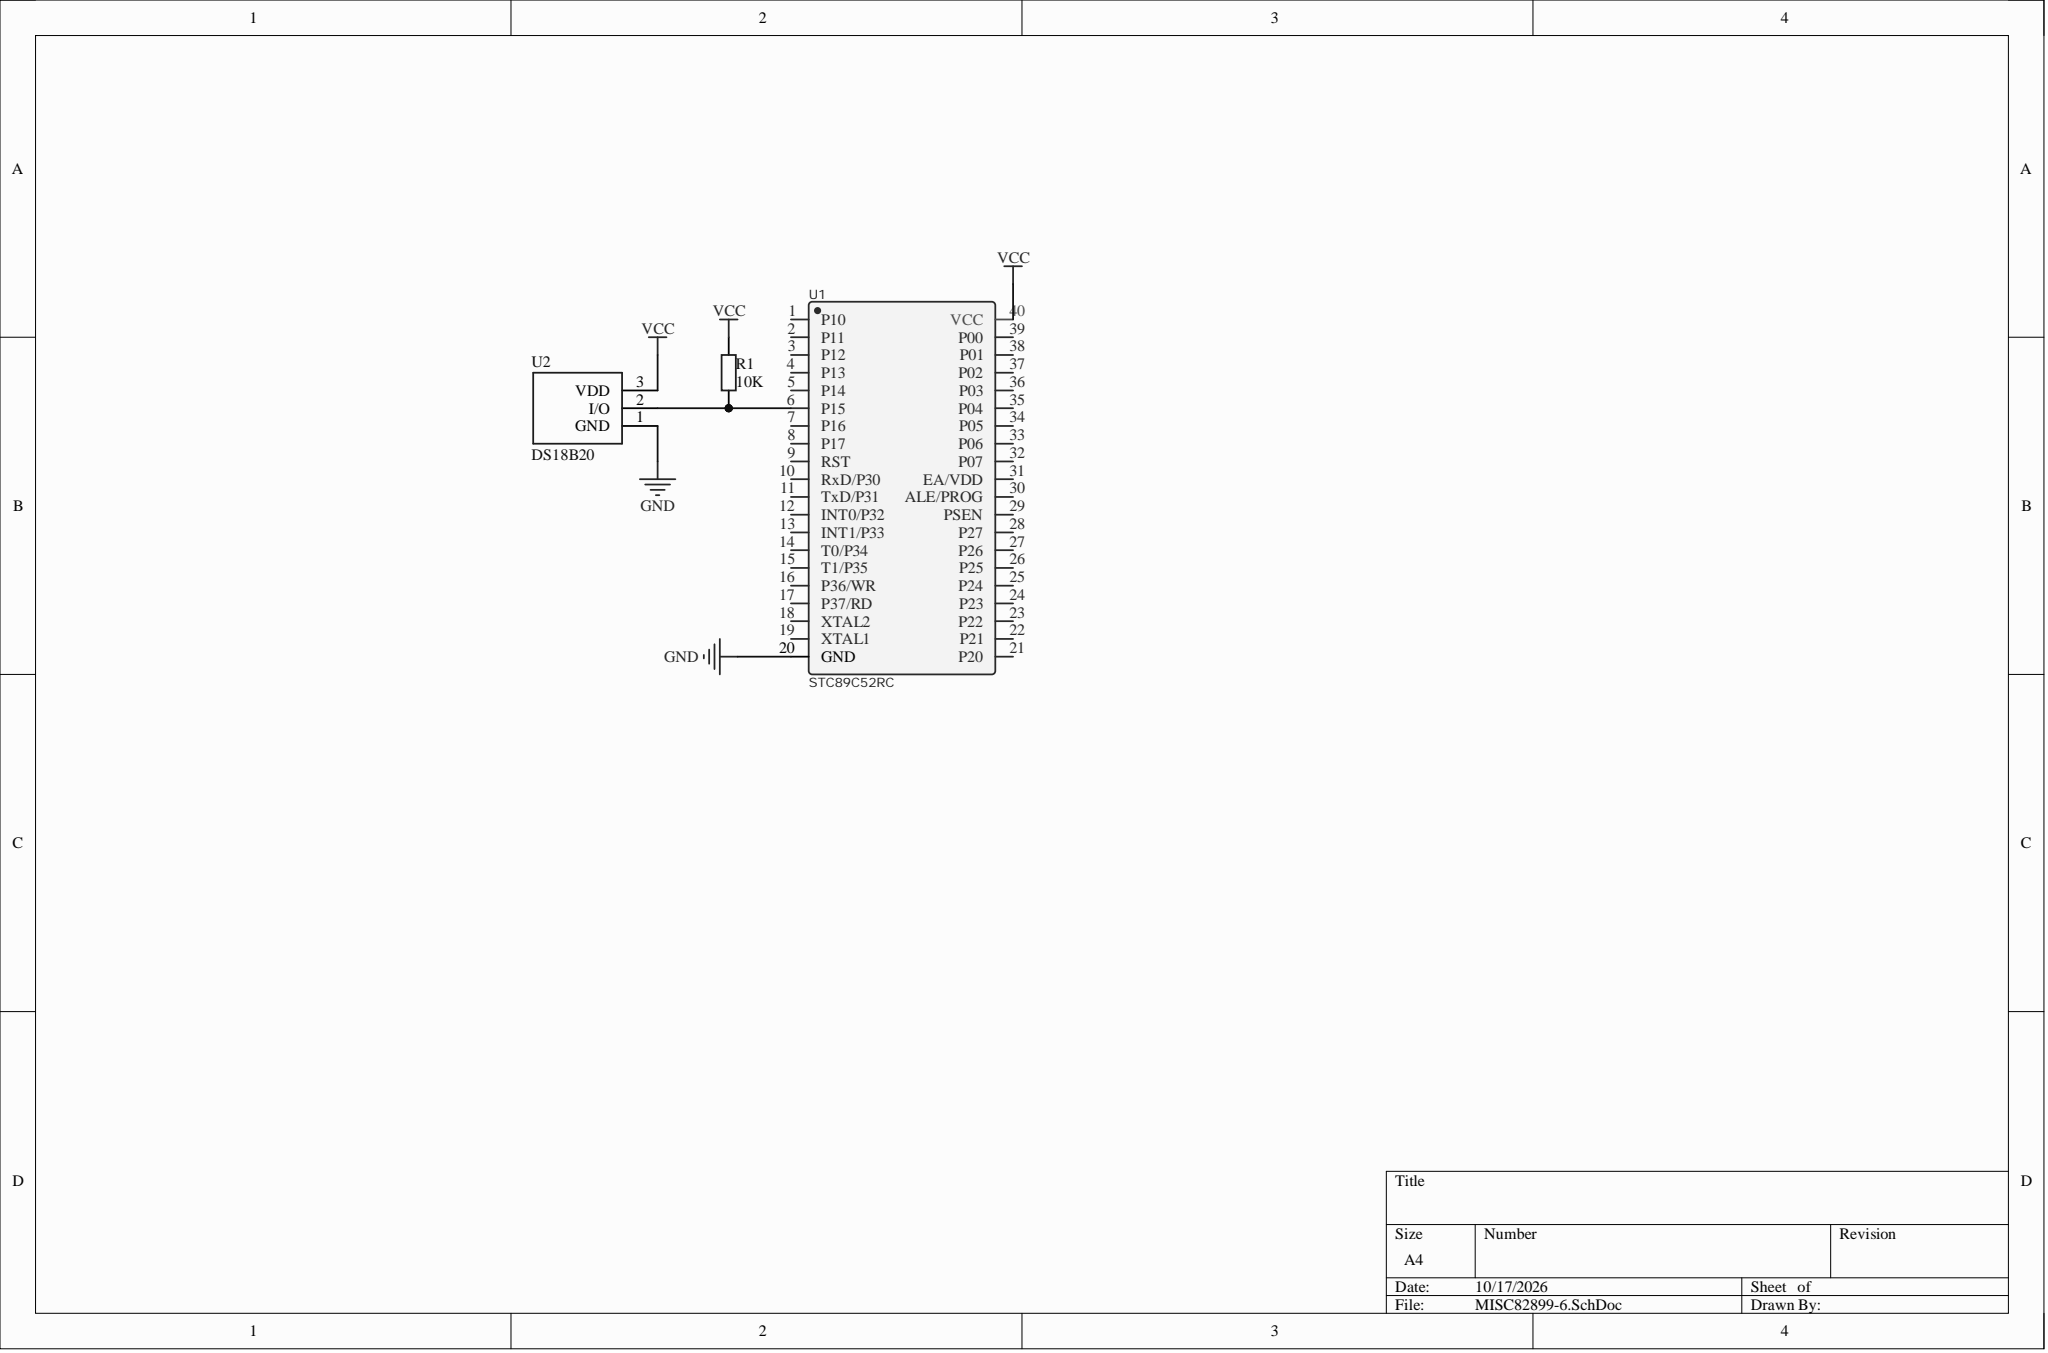Circuit board | Altium Designer | 3 parts | 3 nets
Bill of materials:
Comment,Description,Designator,Footprint,LibRef,Quantity
"10K","Resistor","R1","AXIAL-0.4","Res2","1"
"STC89C52RC","","U1","STC89C52RC","STC89C52RC","1"
"DS18B20","","U2","DS18B20","DS18B20","1"
Netlist (Protel format):
[
R1
AXIAL-0.4
10K



]
[
U1
STC89C52RC
STC89C52RC



]
[
U2
DS18B20
DS18B20



]
(
VCC
R1-2
U1-40
U2-3
)
(
NetR1_1
R1-1
U1-6
U2-2
)
(
GND
U1-20
U2-1
)